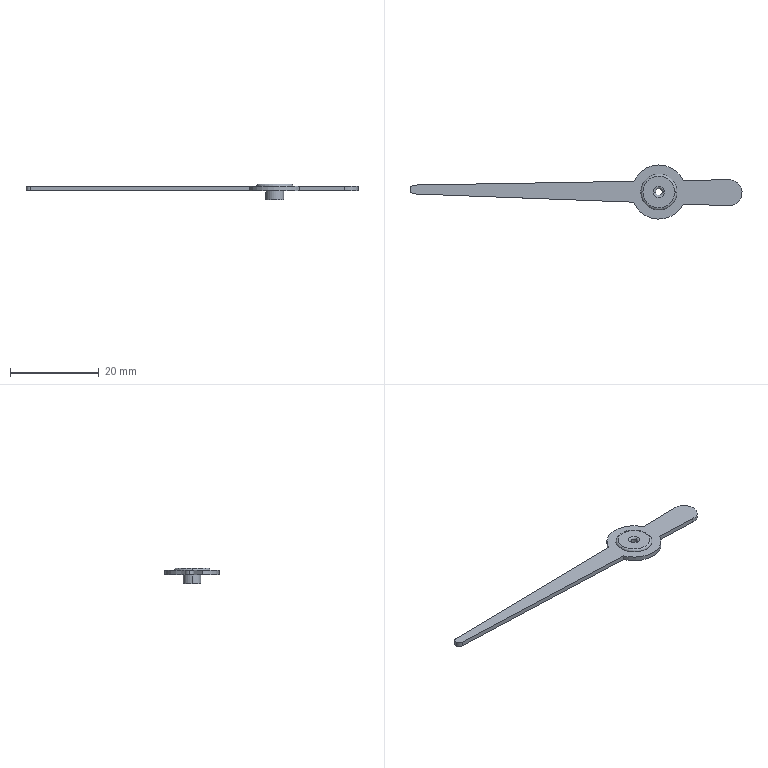Part | SolidWorks | features ICE 4, Extrusion 1, Fillet 1 | 1 solid | 21 faces | box 74.73 x 12.196 x 3.5 mm | volume 394.358 mm3 | cylinder 9 | plane 8 | torus 4 | commonest cylinder face diameters 1.5 x2 2 x2 4 x2 12.196 x2 5.86 x1
STEP:
#1=CARTESIAN_POINT('',(-1.25,0.,1.5));
#2=VERTEX_POINT('',#1);
#3=CARTESIAN_POINT('',(1.25,0.,1.5));
#4=VERTEX_POINT('',#3);
#5=CARTESIAN_POINT('',(0.,0.,1.5));
#6=DIRECTION('',(0.,0.,-1.));
#7=DIRECTION('',(1.,0.,0.));
#8=AXIS2_PLACEMENT_3D('',#5,#6,#7);
#9=CIRCLE('',#8,1.25);
#10=EDGE_CURVE('',#2,#4,#9,.T.);
#11=ORIENTED_EDGE('',*,*,#10,.F.);
#12=CARTESIAN_POINT('',(-0.75,0.,1.));
#13=VERTEX_POINT('',#12);
#14=CARTESIAN_POINT('',(-1.25,0.,1.));
#15=DIRECTION('',(0.,1.,0.));
#16=DIRECTION('',(-1.,0.,0.));
#17=AXIS2_PLACEMENT_3D('',#14,#15,#16);
#18=CIRCLE('',#17,0.5);
#19=EDGE_CURVE('',#2,#13,#18,.T.);
#20=ORIENTED_EDGE('',*,*,#19,.T.);
#21=CARTESIAN_POINT('',(0.75,0.,1.));
#22=VERTEX_POINT('',#21);
#23=CARTESIAN_POINT('',(0.,0.,1.));
#24=DIRECTION('',(0.,0.,1.));
#25=DIRECTION('',(1.,0.,0.));
#26=AXIS2_PLACEMENT_3D('',#23,#24,#25);
#27=CIRCLE('',#26,0.75);
#28=EDGE_CURVE('',#22,#13,#27,.T.);
#29=ORIENTED_EDGE('',*,*,#28,.F.);
#30=CARTESIAN_POINT('',(1.25,0.,1.));
#31=DIRECTION('',(0.,-1.,0.));
#32=DIRECTION('',(0.,0.,-1.));
#33=AXIS2_PLACEMENT_3D('',#30,#31,#32);
#34=CIRCLE('',#33,0.5);
#35=EDGE_CURVE('',#4,#22,#34,.T.);
#36=ORIENTED_EDGE('',*,*,#35,.F.);
#37=EDGE_LOOP('',(#11,#20,#29,#36));
#38=FACE_OUTER_BOUND('',#37,.T.);
#39=CARTESIAN_POINT('',(0.,0.,1.));
#40=DIRECTION('',(0.,0.,1.));
#41=DIRECTION('',(1.,0.,0.));
#42=AXIS2_PLACEMENT_3D('',#39,#40,#41);
#43=TOROIDAL_SURFACE('',#42,1.25,0.5);
#44=ADVANCED_FACE('',(#38),#43,.T.);
#45=CARTESIAN_POINT('',(-4.069,0.,1.));
#46=VERTEX_POINT('',#45);
#47=CARTESIAN_POINT('',(4.069,0.,1.));
#48=VERTEX_POINT('',#47);
#49=CARTESIAN_POINT('',(0.,0.,1.));
#50=DIRECTION('',(0.,0.,-1.));
#51=DIRECTION('',(1.,0.,0.));
#52=AXIS2_PLACEMENT_3D('',#49,#50,#51);
#53=CIRCLE('',#52,4.069);
#54=EDGE_CURVE('',#46,#48,#53,.T.);
#55=ORIENTED_EDGE('',*,*,#54,.F.);
#56=CARTESIAN_POINT('',(-3.569,0.,1.5));
#57=VERTEX_POINT('',#56);
#58=CARTESIAN_POINT('',(-3.569,0.,1.));
#59=DIRECTION('',(0.,1.,0.));
#60=DIRECTION('',(-1.,0.,0.));
#61=AXIS2_PLACEMENT_3D('',#58,#59,#60);
#62=CIRCLE('',#61,0.5);
#63=EDGE_CURVE('',#46,#57,#62,.T.);
#64=ORIENTED_EDGE('',*,*,#63,.T.);
#65=CARTESIAN_POINT('',(3.569,0.,1.5));
#66=VERTEX_POINT('',#65);
#67=CARTESIAN_POINT('',(0.,0.,1.5));
#68=DIRECTION('',(0.,0.,1.));
#69=DIRECTION('',(1.,0.,0.));
#70=AXIS2_PLACEMENT_3D('',#67,#68,#69);
#71=CIRCLE('',#70,3.569);
#72=EDGE_CURVE('',#66,#57,#71,.T.);
#73=ORIENTED_EDGE('',*,*,#72,.F.);
#74=CARTESIAN_POINT('',(3.569,0.,1.));
#75=DIRECTION('',(0.,-1.,0.));
#76=DIRECTION('',(0.,0.,-1.));
#77=AXIS2_PLACEMENT_3D('',#74,#75,#76);
#78=CIRCLE('',#77,0.5);
#79=EDGE_CURVE('',#48,#66,#78,.T.);
#80=ORIENTED_EDGE('',*,*,#79,.F.);
#81=EDGE_LOOP('',(#55,#64,#73,#80));
#82=FACE_OUTER_BOUND('',#81,.T.);
#83=CARTESIAN_POINT('',(0.,0.,1.));
#84=DIRECTION('',(0.,0.,1.));
#85=DIRECTION('',(1.,0.,0.));
#86=AXIS2_PLACEMENT_3D('',#83,#84,#85);
#87=TOROIDAL_SURFACE('',#86,3.569,0.5);
#88=ADVANCED_FACE('',(#82),#87,.T.);
#89=CARTESIAN_POINT('',(-0.75,0.,-2.));
#90=VERTEX_POINT('',#89);
#91=CARTESIAN_POINT('',(0.75,0.,-2.));
#92=VERTEX_POINT('',#91);
#93=CARTESIAN_POINT('',(0.,0.,-2.));
#94=DIRECTION('',(0.,0.,1.));
#95=DIRECTION('',(1.,0.,0.));
#96=AXIS2_PLACEMENT_3D('',#93,#94,#95);
#97=CIRCLE('',#96,0.75);
#98=EDGE_CURVE('',#90,#92,#97,.T.);
#99=ORIENTED_EDGE('',*,*,#98,.F.);
#100=CARTESIAN_POINT('',(-0.75,0.,-2.));
#101=DIRECTION('',(0.,0.,1.));
#102=VECTOR('',#101,1000.);
#103=LINE('',#100,#102);
#104=EDGE_CURVE('',#90,#13,#103,.T.);
#105=ORIENTED_EDGE('',*,*,#104,.T.);
#106=CARTESIAN_POINT('',(0.,0.,1.));
#107=DIRECTION('',(0.,0.,1.));
#108=DIRECTION('',(1.,0.,0.));
#109=AXIS2_PLACEMENT_3D('',#106,#107,#108);
#110=CIRCLE('',#109,0.75);
#111=EDGE_CURVE('',#13,#22,#110,.T.);
#112=ORIENTED_EDGE('',*,*,#111,.T.);
#113=CARTESIAN_POINT('',(0.75,0.,-2.));
#114=DIRECTION('',(0.,0.,1.));
#115=VECTOR('',#114,1000.);
#116=LINE('',#113,#115);
#117=EDGE_CURVE('',#92,#22,#116,.T.);
#118=ORIENTED_EDGE('',*,*,#117,.F.);
#119=EDGE_LOOP('',(#99,#105,#112,#118));
#120=FACE_OUTER_BOUND('',#119,.T.);
#121=CARTESIAN_POINT('',(0.,0.,-2.));
#122=DIRECTION('',(0.,0.,1.));
#123=DIRECTION('',(1.,0.,0.));
#124=AXIS2_PLACEMENT_3D('',#121,#122,#123);
#125=CYLINDRICAL_SURFACE('',#124,0.75);
#126=ADVANCED_FACE('',(#120),#125,.F.);
#127=CARTESIAN_POINT('',(2.,0.,-2.));
#128=VERTEX_POINT('',#127);
#129=CARTESIAN_POINT('',(-2.,0.,-2.));
#130=VERTEX_POINT('',#129);
#131=CARTESIAN_POINT('',(0.,0.,-2.));
#132=DIRECTION('',(0.,0.,1.));
#133=DIRECTION('',(1.,0.,0.));
#134=AXIS2_PLACEMENT_3D('',#131,#132,#133);
#135=CIRCLE('',#134,2.);
#136=EDGE_CURVE('',#128,#130,#135,.T.);
#137=ORIENTED_EDGE('',*,*,#136,.T.);
#138=CARTESIAN_POINT('',(-2.,0.,0.));
#139=VERTEX_POINT('',#138);
#140=CARTESIAN_POINT('',(-2.,0.,-2.));
#141=DIRECTION('',(0.,0.,1.));
#142=VECTOR('',#141,1000.);
#143=LINE('',#140,#142);
#144=EDGE_CURVE('',#130,#139,#143,.T.);
#145=ORIENTED_EDGE('',*,*,#144,.T.);
#146=CARTESIAN_POINT('',(2.,0.,0.));
#147=VERTEX_POINT('',#146);
#148=CARTESIAN_POINT('',(0.,0.,0.));
#149=DIRECTION('',(0.,0.,1.));
#150=DIRECTION('',(1.,0.,0.));
#151=AXIS2_PLACEMENT_3D('',#148,#149,#150);
#152=CIRCLE('',#151,2.);
#153=EDGE_CURVE('',#147,#139,#152,.T.);
#154=ORIENTED_EDGE('',*,*,#153,.F.);
#155=CARTESIAN_POINT('',(2.,0.,-2.));
#156=DIRECTION('',(0.,0.,1.));
#157=VECTOR('',#156,1000.);
#158=LINE('',#155,#157);
#159=EDGE_CURVE('',#128,#147,#158,.T.);
#160=ORIENTED_EDGE('',*,*,#159,.F.);
#161=EDGE_LOOP('',(#137,#145,#154,#160));
#162=FACE_OUTER_BOUND('',#161,.T.);
#163=CARTESIAN_POINT('',(0.,0.,-2.));
#164=DIRECTION('',(0.,0.,1.));
#165=DIRECTION('',(1.,0.,0.));
#166=AXIS2_PLACEMENT_3D('',#163,#164,#165);
#167=CYLINDRICAL_SURFACE('',#166,2.);
#168=ADVANCED_FACE('',(#162),#167,.T.);
#169=CARTESIAN_POINT('',(-56.,0.5656,1.));
#170=VERTEX_POINT('',#169);
#171=CARTESIAN_POINT('',(-55.038,-0.4337,1.));
#172=VERTEX_POINT('',#171);
#173=CARTESIAN_POINT('',(-55.,0.5656,1.));
#174=DIRECTION('',(0.,0.,1.));
#175=DIRECTION('',(1.,0.,0.));
#176=AXIS2_PLACEMENT_3D('',#173,#174,#175);
#177=CIRCLE('',#176,1.);
#178=EDGE_CURVE('',#170,#172,#177,.T.);
#179=ORIENTED_EDGE('',*,*,#178,.F.);
#180=CARTESIAN_POINT('',(-56.,0.5656,0.));
#181=VERTEX_POINT('',#180);
#182=CARTESIAN_POINT('',(-56.,0.5656,1.));
#183=DIRECTION('',(0.,0.,-1.));
#184=VECTOR('',#183,1000.);
#185=LINE('',#182,#184);
#186=EDGE_CURVE('',#170,#181,#185,.T.);
#187=ORIENTED_EDGE('',*,*,#186,.T.);
#188=CARTESIAN_POINT('',(-55.038,-0.4337,0.));
#189=VERTEX_POINT('',#188);
#190=CARTESIAN_POINT('',(-55.,0.5656,0.));
#191=DIRECTION('',(0.,0.,1.));
#192=DIRECTION('',(1.,0.,0.));
#193=AXIS2_PLACEMENT_3D('',#190,#191,#192);
#194=CIRCLE('',#193,1.);
#195=EDGE_CURVE('',#181,#189,#194,.T.);
#196=ORIENTED_EDGE('',*,*,#195,.T.);
#197=CARTESIAN_POINT('',(-55.038,-0.4337,1.));
#198=DIRECTION('',(0.,0.,-1.));
#199=VECTOR('',#198,1000.);
#200=LINE('',#197,#199);
#201=EDGE_CURVE('',#172,#189,#200,.T.);
#202=ORIENTED_EDGE('',*,*,#201,.F.);
#203=EDGE_LOOP('',(#179,#187,#196,#202));
#204=FACE_OUTER_BOUND('',#203,.T.);
#205=CARTESIAN_POINT('',(-55.,0.5656,1.));
#206=DIRECTION('',(0.,0.,-1.));
#207=DIRECTION('',(-1.,0.,0.));
#208=AXIS2_PLACEMENT_3D('',#205,#206,#207);
#209=CYLINDRICAL_SURFACE('',#208,1.);
#210=ADVANCED_FACE('',(#204),#209,.T.);
#211=CARTESIAN_POINT('',(15.75,2.767,0.));
#212=VERTEX_POINT('',#211);
#213=CARTESIAN_POINT('',(15.69,-3.09,0.));
#214=VERTEX_POINT('',#213);
#215=CARTESIAN_POINT('',(15.8,-0.1625,0.));
#216=DIRECTION('',(0.,0.,-1.));
#217=DIRECTION('',(1.,0.,0.));
#218=AXIS2_PLACEMENT_3D('',#215,#216,#217);
#219=CIRCLE('',#218,2.93);
#220=EDGE_CURVE('',#212,#214,#219,.T.);
#221=ORIENTED_EDGE('',*,*,#220,.F.);
#222=CARTESIAN_POINT('',(15.75,2.767,1.));
#223=VERTEX_POINT('',#222);
#224=CARTESIAN_POINT('',(15.75,2.767,1.));
#225=DIRECTION('',(0.,0.,-1.));
#226=VECTOR('',#225,1000.);
#227=LINE('',#224,#226);
#228=EDGE_CURVE('',#223,#212,#227,.T.);
#229=ORIENTED_EDGE('',*,*,#228,.F.);
#230=CARTESIAN_POINT('',(15.69,-3.09,1.));
#231=VERTEX_POINT('',#230);
#232=CARTESIAN_POINT('',(15.8,-0.1625,1.));
#233=DIRECTION('',(0.,0.,-1.));
#234=DIRECTION('',(1.,0.,0.));
#235=AXIS2_PLACEMENT_3D('',#232,#233,#234);
#236=CIRCLE('',#235,2.93);
#237=EDGE_CURVE('',#223,#231,#236,.T.);
#238=ORIENTED_EDGE('',*,*,#237,.T.);
#239=CARTESIAN_POINT('',(15.69,-3.09,1.));
#240=DIRECTION('',(0.,0.,-1.));
#241=VECTOR('',#240,1000.);
#242=LINE('',#239,#241);
#243=EDGE_CURVE('',#231,#214,#242,.T.);
#244=ORIENTED_EDGE('',*,*,#243,.T.);
#245=EDGE_LOOP('',(#221,#229,#238,#244));
#246=FACE_OUTER_BOUND('',#245,.T.);
#247=CARTESIAN_POINT('',(15.8,-0.1625,1.));
#248=DIRECTION('',(0.,0.,-1.));
#249=DIRECTION('',(-1.,0.,0.));
#250=AXIS2_PLACEMENT_3D('',#247,#248,#249);
#251=CYLINDRICAL_SURFACE('',#250,2.93);
#252=ADVANCED_FACE('',(#246),#251,.T.);
#253=CARTESIAN_POINT('',(5.519,2.593,0.));
#254=VERTEX_POINT('',#253);
#255=CARTESIAN_POINT('',(-0.04243,2.499,0.));
#256=DIRECTION('',(-0.9999,-0.01698,0.));
#257=VECTOR('',#256,1000.);
#258=LINE('',#255,#257);
#259=EDGE_CURVE('',#212,#254,#258,.T.);
#260=ORIENTED_EDGE('',*,*,#259,.T.);
#261=CARTESIAN_POINT('',(5.519,2.593,1.));
#262=VERTEX_POINT('',#261);
#263=CARTESIAN_POINT('',(5.519,2.593,1.));
#264=DIRECTION('',(0.,0.,-1.));
#265=VECTOR('',#264,1000.);
#266=LINE('',#263,#265);
#267=EDGE_CURVE('',#262,#254,#266,.T.);
#268=ORIENTED_EDGE('',*,*,#267,.F.);
#269=CARTESIAN_POINT('',(-0.04243,2.499,1.));
#270=DIRECTION('',(-0.9999,-0.01698,0.));
#271=VECTOR('',#270,1000.);
#272=LINE('',#269,#271);
#273=EDGE_CURVE('',#223,#262,#272,.T.);
#274=ORIENTED_EDGE('',*,*,#273,.F.);
#275=ORIENTED_EDGE('',*,*,#228,.T.);
#276=EDGE_LOOP('',(#260,#268,#274,#275));
#277=FACE_OUTER_BOUND('',#276,.T.);
#278=CARTESIAN_POINT('',(-0.04243,2.499,1.));
#279=DIRECTION('',(0.01698,-0.9999,0.));
#280=DIRECTION('',(0.9999,0.01698,0.));
#281=AXIS2_PLACEMENT_3D('',#278,#279,#280);
#282=PLANE('',#281);
#283=ADVANCED_FACE('',(#277),#282,.F.);
#284=CARTESIAN_POINT('',(-5.604,2.405,0.));
#285=VERTEX_POINT('',#284);
#286=CARTESIAN_POINT('',(0.,0.,0.));
#287=DIRECTION('',(0.,0.,1.));
#288=DIRECTION('',(1.,0.,0.));
#289=AXIS2_PLACEMENT_3D('',#286,#287,#288);
#290=CIRCLE('',#289,6.098);
#291=EDGE_CURVE('',#254,#285,#290,.T.);
#292=ORIENTED_EDGE('',*,*,#291,.T.);
#293=CARTESIAN_POINT('',(-5.604,2.405,1.));
#294=VERTEX_POINT('',#293);
#295=CARTESIAN_POINT('',(-5.604,2.405,1.));
#296=DIRECTION('',(0.,0.,-1.));
#297=VECTOR('',#296,1000.);
#298=LINE('',#295,#297);
#299=EDGE_CURVE('',#294,#285,#298,.T.);
#300=ORIENTED_EDGE('',*,*,#299,.F.);
#301=CARTESIAN_POINT('',(0.,0.,1.));
#302=DIRECTION('',(0.,0.,1.));
#303=DIRECTION('',(1.,0.,0.));
#304=AXIS2_PLACEMENT_3D('',#301,#302,#303);
#305=CIRCLE('',#304,6.098);
#306=EDGE_CURVE('',#262,#294,#305,.T.);
#307=ORIENTED_EDGE('',*,*,#306,.F.);
#308=ORIENTED_EDGE('',*,*,#267,.T.);
#309=EDGE_LOOP('',(#292,#300,#307,#308));
#310=FACE_OUTER_BOUND('',#309,.T.);
#311=CARTESIAN_POINT('',(0.,0.,1.));
#312=DIRECTION('',(0.,0.,-1.));
#313=DIRECTION('',(-1.,0.,0.));
#314=AXIS2_PLACEMENT_3D('',#311,#312,#313);
#315=CYLINDRICAL_SURFACE('',#314,6.098);
#316=ADVANCED_FACE('',(#310),#315,.T.);
#317=CARTESIAN_POINT('',(-55.017,1.565,0.));
#318=VERTEX_POINT('',#317);
#319=CARTESIAN_POINT('',(-0.04243,2.499,0.));
#320=DIRECTION('',(-0.9999,-0.01698,0.));
#321=VECTOR('',#320,1000.);
#322=LINE('',#319,#321);
#323=EDGE_CURVE('',#285,#318,#322,.T.);
#324=ORIENTED_EDGE('',*,*,#323,.T.);
#325=CARTESIAN_POINT('',(-55.017,1.565,1.));
#326=VERTEX_POINT('',#325);
#327=CARTESIAN_POINT('',(-55.017,1.565,1.));
#328=DIRECTION('',(0.,0.,-1.));
#329=VECTOR('',#328,1000.);
#330=LINE('',#327,#329);
#331=EDGE_CURVE('',#326,#318,#330,.T.);
#332=ORIENTED_EDGE('',*,*,#331,.F.);
#333=CARTESIAN_POINT('',(-0.04243,2.499,1.));
#334=DIRECTION('',(-0.9999,-0.01698,0.));
#335=VECTOR('',#334,1000.);
#336=LINE('',#333,#335);
#337=EDGE_CURVE('',#294,#326,#336,.T.);
#338=ORIENTED_EDGE('',*,*,#337,.F.);
#339=ORIENTED_EDGE('',*,*,#299,.T.);
#340=EDGE_LOOP('',(#324,#332,#338,#339));
#341=FACE_OUTER_BOUND('',#340,.T.);
#342=CARTESIAN_POINT('',(-0.04243,2.499,1.));
#343=DIRECTION('',(0.01698,-0.9999,0.));
#344=DIRECTION('',(0.9999,0.01698,0.));
#345=AXIS2_PLACEMENT_3D('',#342,#343,#344);
#346=PLANE('',#345);
#347=ADVANCED_FACE('',(#341),#346,.F.);
#348=ORIENTED_EDGE('',*,*,#186,.F.);
#349=CARTESIAN_POINT('',(-55.,0.5656,1.));
#350=DIRECTION('',(0.,0.,1.));
#351=DIRECTION('',(1.,0.,0.));
#352=AXIS2_PLACEMENT_3D('',#349,#350,#351);
#353=CIRCLE('',#352,1.);
#354=EDGE_CURVE('',#326,#170,#353,.T.);
#355=ORIENTED_EDGE('',*,*,#354,.F.);
#356=ORIENTED_EDGE('',*,*,#331,.T.);
#357=CARTESIAN_POINT('',(-55.,0.5656,0.));
#358=DIRECTION('',(0.,0.,1.));
#359=DIRECTION('',(1.,0.,0.));
#360=AXIS2_PLACEMENT_3D('',#357,#358,#359);
#361=CIRCLE('',#360,1.);
#362=EDGE_CURVE('',#318,#181,#361,.T.);
#363=ORIENTED_EDGE('',*,*,#362,.T.);
#364=EDGE_LOOP('',(#348,#355,#356,#363));
#365=FACE_OUTER_BOUND('',#364,.T.);
#366=CARTESIAN_POINT('',(-55.,0.5656,1.));
#367=DIRECTION('',(0.,0.,-1.));
#368=DIRECTION('',(-1.,0.,0.));
#369=AXIS2_PLACEMENT_3D('',#366,#367,#368);
#370=CYLINDRICAL_SURFACE('',#369,1.);
#371=ADVANCED_FACE('',(#365),#370,.T.);
#372=CARTESIAN_POINT('',(-5.652,-2.289,0.));
#373=VERTEX_POINT('',#372);
#374=CARTESIAN_POINT('',(-0.09382,-2.498,0.));
#375=DIRECTION('',(0.9993,-0.03754,0.));
#376=VECTOR('',#375,1000.);
#377=LINE('',#374,#376);
#378=EDGE_CURVE('',#189,#373,#377,.T.);
#379=ORIENTED_EDGE('',*,*,#378,.T.);
#380=CARTESIAN_POINT('',(-5.652,-2.289,1.));
#381=VERTEX_POINT('',#380);
#382=CARTESIAN_POINT('',(-5.652,-2.289,1.));
#383=DIRECTION('',(0.,0.,-1.));
#384=VECTOR('',#383,1000.);
#385=LINE('',#382,#384);
#386=EDGE_CURVE('',#381,#373,#385,.T.);
#387=ORIENTED_EDGE('',*,*,#386,.F.);
#388=CARTESIAN_POINT('',(-0.09382,-2.498,1.));
#389=DIRECTION('',(0.9993,-0.03754,0.));
#390=VECTOR('',#389,1000.);
#391=LINE('',#388,#390);
#392=EDGE_CURVE('',#172,#381,#391,.T.);
#393=ORIENTED_EDGE('',*,*,#392,.F.);
#394=ORIENTED_EDGE('',*,*,#201,.T.);
#395=EDGE_LOOP('',(#379,#387,#393,#394));
#396=FACE_OUTER_BOUND('',#395,.T.);
#397=CARTESIAN_POINT('',(-0.09382,-2.498,1.));
#398=DIRECTION('',(0.03754,0.9993,0.));
#399=DIRECTION('',(-0.9993,0.03754,0.));
#400=AXIS2_PLACEMENT_3D('',#397,#398,#399);
#401=PLANE('',#400);
#402=ADVANCED_FACE('',(#396),#401,.F.);
#403=CARTESIAN_POINT('',(5.464,-2.706,0.));
#404=VERTEX_POINT('',#403);
#405=CARTESIAN_POINT('',(0.,0.,0.));
#406=DIRECTION('',(0.,0.,1.));
#407=DIRECTION('',(1.,0.,0.));
#408=AXIS2_PLACEMENT_3D('',#405,#406,#407);
#409=CIRCLE('',#408,6.098);
#410=EDGE_CURVE('',#373,#404,#409,.T.);
#411=ORIENTED_EDGE('',*,*,#410,.T.);
#412=CARTESIAN_POINT('',(5.464,-2.706,1.));
#413=VERTEX_POINT('',#412);
#414=CARTESIAN_POINT('',(5.464,-2.706,1.));
#415=DIRECTION('',(0.,0.,-1.));
#416=VECTOR('',#415,1000.);
#417=LINE('',#414,#416);
#418=EDGE_CURVE('',#413,#404,#417,.T.);
#419=ORIENTED_EDGE('',*,*,#418,.F.);
#420=CARTESIAN_POINT('',(0.,0.,1.));
#421=DIRECTION('',(0.,0.,1.));
#422=DIRECTION('',(1.,0.,0.));
#423=AXIS2_PLACEMENT_3D('',#420,#421,#422);
#424=CIRCLE('',#423,6.098);
#425=EDGE_CURVE('',#381,#413,#424,.T.);
#426=ORIENTED_EDGE('',*,*,#425,.F.);
#427=ORIENTED_EDGE('',*,*,#386,.T.);
#428=EDGE_LOOP('',(#411,#419,#426,#427));
#429=FACE_OUTER_BOUND('',#428,.T.);
#430=CARTESIAN_POINT('',(0.,0.,1.));
#431=DIRECTION('',(0.,0.,-1.));
#432=DIRECTION('',(-1.,0.,0.));
#433=AXIS2_PLACEMENT_3D('',#430,#431,#432);
#434=CYLINDRICAL_SURFACE('',#433,6.098);
#435=ADVANCED_FACE('',(#429),#434,.T.);
#436=CARTESIAN_POINT('',(-0.09382,-2.498,0.));
#437=DIRECTION('',(0.9993,-0.03754,0.));
#438=VECTOR('',#437,1000.);
#439=LINE('',#436,#438);
#440=EDGE_CURVE('',#404,#214,#439,.T.);
#441=ORIENTED_EDGE('',*,*,#440,.T.);
#442=ORIENTED_EDGE('',*,*,#243,.F.);
#443=CARTESIAN_POINT('',(-0.09382,-2.498,1.));
#444=DIRECTION('',(0.9993,-0.03754,0.));
#445=VECTOR('',#444,1000.);
#446=LINE('',#443,#445);
#447=EDGE_CURVE('',#413,#231,#446,.T.);
#448=ORIENTED_EDGE('',*,*,#447,.F.);
#449=ORIENTED_EDGE('',*,*,#418,.T.);
#450=EDGE_LOOP('',(#441,#442,#448,#449));
#451=FACE_OUTER_BOUND('',#450,.T.);
#452=CARTESIAN_POINT('',(-0.09382,-2.498,1.));
#453=DIRECTION('',(0.03754,0.9993,0.));
#454=DIRECTION('',(-0.9993,0.03754,0.));
#455=AXIS2_PLACEMENT_3D('',#452,#453,#454);
#456=PLANE('',#455);
#457=ADVANCED_FACE('',(#451),#456,.F.);
#458=CARTESIAN_POINT('',(0.,0.,1.));
#459=DIRECTION('',(0.,0.,-1.));
#460=DIRECTION('',(1.,0.,0.));
#461=AXIS2_PLACEMENT_3D('',#458,#459,#460);
#462=CIRCLE('',#461,4.069);
#463=EDGE_CURVE('',#48,#46,#462,.T.);
#464=ORIENTED_EDGE('',*,*,#463,.T.);
#465=ORIENTED_EDGE('',*,*,#54,.T.);
#466=EDGE_LOOP('',(#464,#465));
#467=FACE_BOUND('',#466,.T.);
#468=ORIENTED_EDGE('',*,*,#237,.F.);
#469=ORIENTED_EDGE('',*,*,#273,.T.);
#470=ORIENTED_EDGE('',*,*,#306,.T.);
#471=ORIENTED_EDGE('',*,*,#337,.T.);
#472=ORIENTED_EDGE('',*,*,#354,.T.);
#473=ORIENTED_EDGE('',*,*,#178,.T.);
#474=ORIENTED_EDGE('',*,*,#392,.T.);
#475=ORIENTED_EDGE('',*,*,#425,.T.);
#476=ORIENTED_EDGE('',*,*,#447,.T.);
#477=EDGE_LOOP('',(#468,#469,#470,#471,#472,#473,#474,#475,#476));
#478=FACE_OUTER_BOUND('',#477,.T.);
#479=CARTESIAN_POINT('',(0.,0.,1.));
#480=DIRECTION('',(0.,0.,1.));
#481=DIRECTION('',(1.,0.,0.));
#482=AXIS2_PLACEMENT_3D('',#479,#480,#481);
#483=PLANE('',#482);
#484=ADVANCED_FACE('',(#467,#478),#483,.T.);
#485=ORIENTED_EDGE('',*,*,#220,.T.);
#486=ORIENTED_EDGE('',*,*,#440,.F.);
#487=ORIENTED_EDGE('',*,*,#410,.F.);
#488=ORIENTED_EDGE('',*,*,#378,.F.);
#489=ORIENTED_EDGE('',*,*,#195,.F.);
#490=ORIENTED_EDGE('',*,*,#362,.F.);
#491=ORIENTED_EDGE('',*,*,#323,.F.);
#492=ORIENTED_EDGE('',*,*,#291,.F.);
#493=ORIENTED_EDGE('',*,*,#259,.F.);
#494=EDGE_LOOP('',(#485,#486,#487,#488,#489,#490,#491,#492,#493));
#495=FACE_OUTER_BOUND('',#494,.T.);
#496=ORIENTED_EDGE('',*,*,#153,.T.);
#497=CARTESIAN_POINT('',(0.,0.,0.));
#498=DIRECTION('',(0.,0.,1.));
#499=DIRECTION('',(1.,0.,0.));
#500=AXIS2_PLACEMENT_3D('',#497,#498,#499);
#501=CIRCLE('',#500,2.);
#502=EDGE_CURVE('',#139,#147,#501,.T.);
#503=ORIENTED_EDGE('',*,*,#502,.T.);
#504=EDGE_LOOP('',(#496,#503));
#505=FACE_BOUND('',#504,.T.);
#506=CARTESIAN_POINT('',(0.,0.,0.));
#507=DIRECTION('',(0.,0.,1.));
#508=DIRECTION('',(1.,0.,0.));
#509=AXIS2_PLACEMENT_3D('',#506,#507,#508);
#510=PLANE('',#509);
#511=ADVANCED_FACE('',(#495,#505),#510,.F.);
#512=ORIENTED_EDGE('',*,*,#144,.F.);
#513=CARTESIAN_POINT('',(0.,0.,-2.));
#514=DIRECTION('',(0.,0.,1.));
#515=DIRECTION('',(1.,0.,0.));
#516=AXIS2_PLACEMENT_3D('',#513,#514,#515);
#517=CIRCLE('',#516,2.);
#518=EDGE_CURVE('',#130,#128,#517,.T.);
#519=ORIENTED_EDGE('',*,*,#518,.T.);
#520=ORIENTED_EDGE('',*,*,#159,.T.);
#521=ORIENTED_EDGE('',*,*,#502,.F.);
#522=EDGE_LOOP('',(#512,#519,#520,#521));
#523=FACE_OUTER_BOUND('',#522,.T.);
#524=CARTESIAN_POINT('',(0.,0.,-2.));
#525=DIRECTION('',(0.,0.,1.));
#526=DIRECTION('',(1.,0.,0.));
#527=AXIS2_PLACEMENT_3D('',#524,#525,#526);
#528=CYLINDRICAL_SURFACE('',#527,2.);
#529=ADVANCED_FACE('',(#523),#528,.T.);
#530=CARTESIAN_POINT('',(0.,0.,-2.));
#531=DIRECTION('',(0.,0.,1.));
#532=DIRECTION('',(1.,0.,0.));
#533=AXIS2_PLACEMENT_3D('',#530,#531,#532);
#534=CIRCLE('',#533,0.75);
#535=EDGE_CURVE('',#92,#90,#534,.T.);
#536=ORIENTED_EDGE('',*,*,#535,.T.);
#537=ORIENTED_EDGE('',*,*,#98,.T.);
#538=EDGE_LOOP('',(#536,#537));
#539=FACE_BOUND('',#538,.T.);
#540=ORIENTED_EDGE('',*,*,#136,.F.);
#541=ORIENTED_EDGE('',*,*,#518,.F.);
#542=EDGE_LOOP('',(#540,#541));
#543=FACE_OUTER_BOUND('',#542,.T.);
#544=CARTESIAN_POINT('',(0.,0.,-2.));
#545=DIRECTION('',(0.,0.,1.));
#546=DIRECTION('',(1.,0.,0.));
#547=AXIS2_PLACEMENT_3D('',#544,#545,#546);
#548=PLANE('',#547);
#549=ADVANCED_FACE('',(#539,#543),#548,.F.);
#550=ORIENTED_EDGE('',*,*,#72,.T.);
#551=CARTESIAN_POINT('',(0.,0.,1.5));
#552=DIRECTION('',(0.,0.,1.));
#553=DIRECTION('',(1.,0.,0.));
#554=AXIS2_PLACEMENT_3D('',#551,#552,#553);
#555=CIRCLE('',#554,3.569);
#556=EDGE_CURVE('',#57,#66,#555,.T.);
#557=ORIENTED_EDGE('',*,*,#556,.T.);
#558=EDGE_LOOP('',(#550,#557));
#559=FACE_OUTER_BOUND('',#558,.T.);
#560=CARTESIAN_POINT('',(0.,0.,1.5));
#561=DIRECTION('',(0.,0.,-1.));
#562=DIRECTION('',(1.,0.,0.));
#563=AXIS2_PLACEMENT_3D('',#560,#561,#562);
#564=CIRCLE('',#563,1.25);
#565=EDGE_CURVE('',#4,#2,#564,.T.);
#566=ORIENTED_EDGE('',*,*,#565,.T.);
#567=ORIENTED_EDGE('',*,*,#10,.T.);
#568=EDGE_LOOP('',(#566,#567));
#569=FACE_BOUND('',#568,.T.);
#570=CARTESIAN_POINT('',(0.,0.,1.5));
#571=DIRECTION('',(0.,0.,1.));
#572=DIRECTION('',(1.,0.,0.));
#573=AXIS2_PLACEMENT_3D('',#570,#571,#572);
#574=PLANE('',#573);
#575=ADVANCED_FACE('',(#559,#569),#574,.T.);
#576=ORIENTED_EDGE('',*,*,#104,.F.);
#577=ORIENTED_EDGE('',*,*,#535,.F.);
#578=ORIENTED_EDGE('',*,*,#117,.T.);
#579=ORIENTED_EDGE('',*,*,#28,.T.);
#580=EDGE_LOOP('',(#576,#577,#578,#579));
#581=FACE_OUTER_BOUND('',#580,.T.);
#582=CARTESIAN_POINT('',(0.,0.,-2.));
#583=DIRECTION('',(0.,0.,1.));
#584=DIRECTION('',(1.,0.,0.));
#585=AXIS2_PLACEMENT_3D('',#582,#583,#584);
#586=CYLINDRICAL_SURFACE('',#585,0.75);
#587=ADVANCED_FACE('',(#581),#586,.F.);
#588=ORIENTED_EDGE('',*,*,#63,.F.);
#589=ORIENTED_EDGE('',*,*,#463,.F.);
#590=ORIENTED_EDGE('',*,*,#79,.T.);
#591=ORIENTED_EDGE('',*,*,#556,.F.);
#592=EDGE_LOOP('',(#588,#589,#590,#591));
#593=FACE_OUTER_BOUND('',#592,.T.);
#594=CARTESIAN_POINT('',(0.,0.,1.));
#595=DIRECTION('',(0.,0.,1.));
#596=DIRECTION('',(1.,0.,0.));
#597=AXIS2_PLACEMENT_3D('',#594,#595,#596);
#598=TOROIDAL_SURFACE('',#597,3.569,0.5);
#599=ADVANCED_FACE('',(#593),#598,.T.);
#600=ORIENTED_EDGE('',*,*,#19,.F.);
#601=ORIENTED_EDGE('',*,*,#565,.F.);
#602=ORIENTED_EDGE('',*,*,#35,.T.);
#603=ORIENTED_EDGE('',*,*,#111,.F.);
#604=EDGE_LOOP('',(#600,#601,#602,#603));
#605=FACE_OUTER_BOUND('',#604,.T.);
#606=CARTESIAN_POINT('',(0.,0.,1.));
#607=DIRECTION('',(0.,0.,1.));
#608=DIRECTION('',(1.,0.,0.));
#609=AXIS2_PLACEMENT_3D('',#606,#607,#608);
#610=TOROIDAL_SURFACE('',#609,1.25,0.5);
#611=ADVANCED_FACE('',(#605),#610,.T.);
#612=CLOSED_SHELL('',(#44,#88,#126,#168,#210,#252,#283,#316,#347,#371,#402,#435,#457,#484,#511,#529,#549,#575,#587,#599,#611));
#613=MANIFOLD_SOLID_BREP('',#612);
#614=CARTESIAN_POINT('',(0.,0.,0.));
#615=DIRECTION('',(0.,0.,1.));
#616=DIRECTION('',(1.,0.,0.));
#617=AXIS2_PLACEMENT_3D('',#614,#615,#616);
#618=(LENGTH_UNIT()NAMED_UNIT(*)SI_UNIT(.MILLI.,.METRE.));
#619=UNCERTAINTY_MEASURE_WITH_UNIT(LENGTH_MEASURE(0.00001),#618,'','');
#620=(NAMED_UNIT(*)PLANE_ANGLE_UNIT()SI_UNIT($,.RADIAN.));
#621=(NAMED_UNIT(*)SI_UNIT($,.STERADIAN.)SOLID_ANGLE_UNIT());
#622=(GEOMETRIC_REPRESENTATION_CONTEXT(3)GLOBAL_UNCERTAINTY_ASSIGNED_CONTEXT((#619))GLOBAL_UNIT_ASSIGNED_CONTEXT((#618,#620,#621))REPRESENTATION_CONTEXT('',''));
#623=ADVANCED_BREP_SHAPE_REPRESENTATION('',(#613,#617),#622);